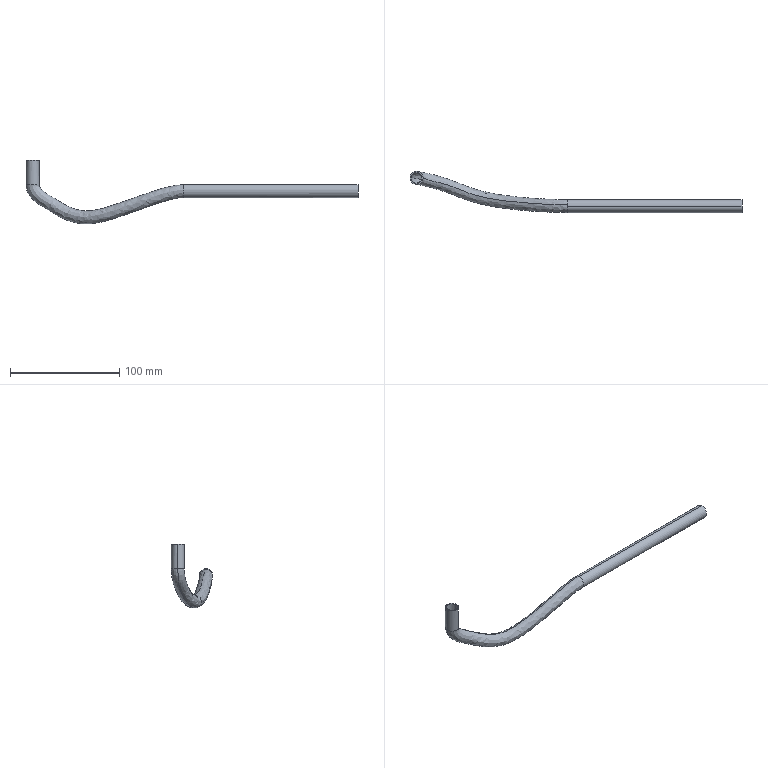Part | SolidWorks | features 3DProfileFeature 2, Sweep 1 | 1 solid | 14 faces | box 304.477 x 37.845 x 58.68 mm | volume 11725 mm3 | cylinder 8 | spline 4 | plane 2 | commonest cylinder face diameters 10 x4 12 x4